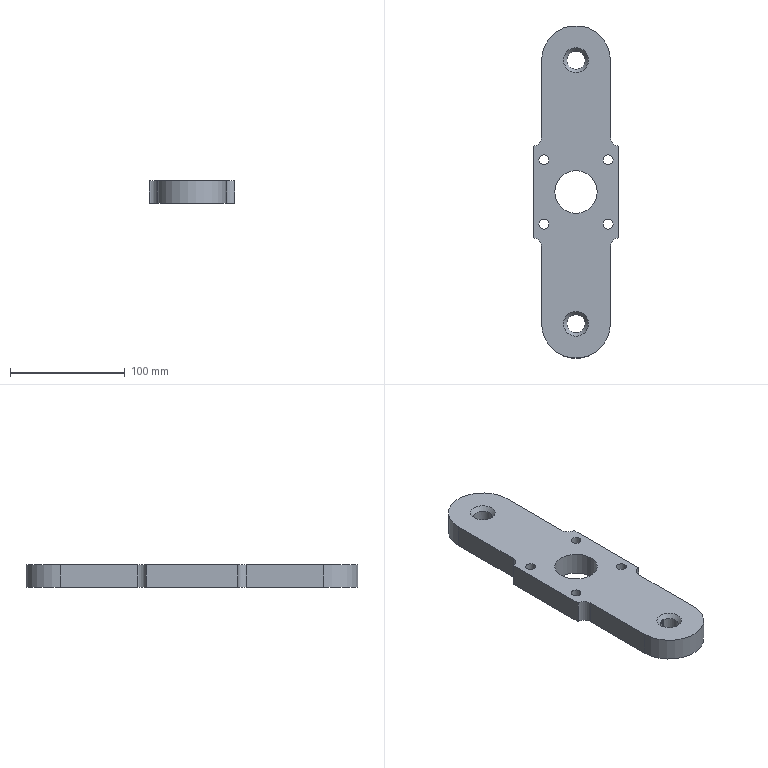Part | STEP file | YBQDJ-QD-10 | 1 solid | 37 faces | box 75 x 290 x 20 mm | volume 318824 mm3 | cylinder 23 | plane 12 | cone 2 | commonest cylinder face diameters 4 x4 8.7 x4 14 x4 15 x4 1 x2 16 x2